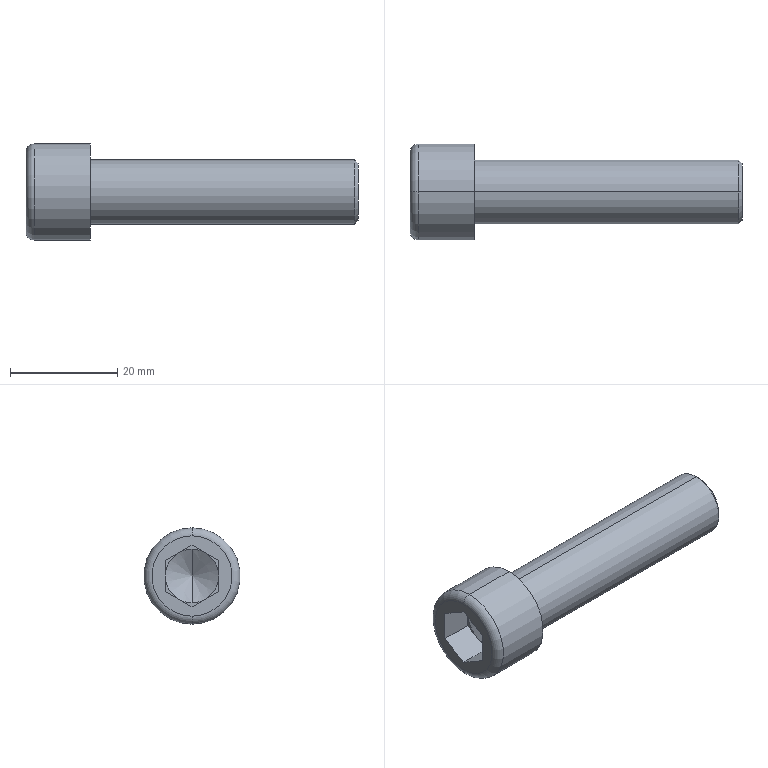Part | STEP file | hexagon socket head cap screws gb_GB_FASTENER_SCREWS_HSHCS M12X50-N | 1 solid | 25 faces | box 62 x 18 x 18 mm | volume 8080 mm3 | plane 15 | cone 4 | cylinder 4 | torus 2 | commonest cylinder face diameters 12 x2 18 x2
STEP:
#1=CARTESIAN_POINT('',(62.,0.,-5.4));
#2=VERTEX_POINT('',#1);
#3=CARTESIAN_POINT('',(62.,0.,5.4));
#4=VERTEX_POINT('',#3);
#5=CARTESIAN_POINT('',(62.,0.,0.));
#6=DIRECTION('',(1.,0.,0.));
#7=DIRECTION('',(0.,0.,-1.));
#8=AXIS2_PLACEMENT_3D('',#5,#6,#7);
#9=CIRCLE('',#8,5.4);
#10=EDGE_CURVE('',#2,#4,#9,.T.);
#11=ORIENTED_EDGE('',*,*,#10,.F.);
#12=CARTESIAN_POINT('',(61.4,0.,-6.));
#13=VERTEX_POINT('',#12);
#14=CARTESIAN_POINT('',(62.,0.,-5.4));
#15=DIRECTION('',(-0.7071,0.,-0.7071));
#16=VECTOR('',#15,1000.);
#17=LINE('',#14,#16);
#18=EDGE_CURVE('',#2,#13,#17,.T.);
#19=ORIENTED_EDGE('',*,*,#18,.T.);
#20=CARTESIAN_POINT('',(61.4,0.,6.));
#21=VERTEX_POINT('',#20);
#22=CARTESIAN_POINT('',(61.4,0.,0.));
#23=DIRECTION('',(-1.,0.,0.));
#24=DIRECTION('',(0.,0.,-1.));
#25=AXIS2_PLACEMENT_3D('',#22,#23,#24);
#26=CIRCLE('',#25,6.);
#27=EDGE_CURVE('',#21,#13,#26,.T.);
#28=ORIENTED_EDGE('',*,*,#27,.F.);
#29=CARTESIAN_POINT('',(62.,0.,5.4));
#30=DIRECTION('',(-0.7071,0.,0.7071));
#31=VECTOR('',#30,1000.);
#32=LINE('',#29,#31);
#33=EDGE_CURVE('',#4,#21,#32,.T.);
#34=ORIENTED_EDGE('',*,*,#33,.F.);
#35=EDGE_LOOP('',(#11,#19,#28,#34));
#36=FACE_OUTER_BOUND('',#35,.T.);
#37=CARTESIAN_POINT('',(62.,0.,0.));
#38=DIRECTION('',(-1.,0.,0.));
#39=DIRECTION('',(0.,0.,1.));
#40=AXIS2_PLACEMENT_3D('',#37,#38,#39);
#41=CONICAL_SURFACE('',#40,5.4,0.7854);
#42=ADVANCED_FACE('',(#36),#41,.T.);
#43=CARTESIAN_POINT('',(0.,0.,7.5));
#44=VERTEX_POINT('',#43);
#45=CARTESIAN_POINT('',(0.,0.,-7.5));
#46=VERTEX_POINT('',#45);
#47=CARTESIAN_POINT('',(0.,0.,0.));
#48=DIRECTION('',(-1.,0.,0.));
#49=DIRECTION('',(0.,0.,-1.));
#50=AXIS2_PLACEMENT_3D('',#47,#48,#49);
#51=CIRCLE('',#50,7.5);
#52=EDGE_CURVE('',#44,#46,#51,.T.);
#53=ORIENTED_EDGE('',*,*,#52,.F.);
#54=CARTESIAN_POINT('',(1.5,0.,9.));
#55=VERTEX_POINT('',#54);
#56=CARTESIAN_POINT('',(1.5,0.,7.5));
#57=DIRECTION('',(0.,1.,0.));
#58=DIRECTION('',(0.,0.,1.));
#59=AXIS2_PLACEMENT_3D('',#56,#57,#58);
#60=CIRCLE('',#59,1.5);
#61=EDGE_CURVE('',#44,#55,#60,.T.);
#62=ORIENTED_EDGE('',*,*,#61,.T.);
#63=CARTESIAN_POINT('',(1.5,0.,-9.));
#64=VERTEX_POINT('',#63);
#65=CARTESIAN_POINT('',(1.5,0.,0.));
#66=DIRECTION('',(1.,0.,0.));
#67=DIRECTION('',(0.,0.,-1.));
#68=AXIS2_PLACEMENT_3D('',#65,#66,#67);
#69=CIRCLE('',#68,9.);
#70=EDGE_CURVE('',#64,#55,#69,.T.);
#71=ORIENTED_EDGE('',*,*,#70,.F.);
#72=CARTESIAN_POINT('',(1.5,0.,-7.5));
#73=DIRECTION('',(0.,-1.,0.));
#74=DIRECTION('',(0.,0.,-1.));
#75=AXIS2_PLACEMENT_3D('',#72,#73,#74);
#76=CIRCLE('',#75,1.5);
#77=EDGE_CURVE('',#46,#64,#76,.T.);
#78=ORIENTED_EDGE('',*,*,#77,.F.);
#79=EDGE_LOOP('',(#53,#62,#71,#78));
#80=FACE_OUTER_BOUND('',#79,.T.);
#81=CARTESIAN_POINT('',(1.5,0.,0.));
#82=DIRECTION('',(1.,0.,0.));
#83=DIRECTION('',(0.,0.,-1.));
#84=AXIS2_PLACEMENT_3D('',#81,#82,#83);
#85=TOROIDAL_SURFACE('',#84,7.5,1.5);
#86=ADVANCED_FACE('',(#80),#85,.T.);
#87=CARTESIAN_POINT('',(8.887,0.,0.));
#88=VERTEX_POINT('',#87);
#89=CARTESIAN_POINT('',(6.,0.,5.));
#90=VERTEX_POINT('',#89);
#91=CARTESIAN_POINT('',(6.,0.,5.));
#92=DIRECTION('',(-0.5,0.,0.866));
#93=VECTOR('',#92,1000.);
#94=LINE('',#91,#93);
#95=EDGE_CURVE('',#88,#90,#94,.T.);
#96=ORIENTED_EDGE('',*,*,#95,.F.);
#97=CARTESIAN_POINT('',(6.,0.,-5.));
#98=VERTEX_POINT('',#97);
#99=CARTESIAN_POINT('',(6.,0.,-5.));
#100=DIRECTION('',(-0.5,0.,-0.866));
#101=VECTOR('',#100,1000.);
#102=LINE('',#99,#101);
#103=EDGE_CURVE('',#88,#98,#102,.T.);
#104=ORIENTED_EDGE('',*,*,#103,.T.);
#105=CARTESIAN_POINT('',(6.,-2.5,-4.33));
#106=VERTEX_POINT('',#105);
#107=CARTESIAN_POINT('',(6.,0.,0.));
#108=DIRECTION('',(-1.,0.,0.));
#109=DIRECTION('',(0.,0.,-1.));
#110=AXIS2_PLACEMENT_3D('',#107,#108,#109);
#111=CIRCLE('',#110,5.);
#112=EDGE_CURVE('',#98,#106,#111,.T.);
#113=ORIENTED_EDGE('',*,*,#112,.T.);
#114=CARTESIAN_POINT('',(6.,-5.,0.));
#115=VERTEX_POINT('',#114);
#116=CARTESIAN_POINT('',(6.,0.,0.));
#117=DIRECTION('',(-1.,0.,0.));
#118=DIRECTION('',(0.,0.,-1.));
#119=AXIS2_PLACEMENT_3D('',#116,#117,#118);
#120=CIRCLE('',#119,5.);
#121=EDGE_CURVE('',#106,#115,#120,.T.);
#122=ORIENTED_EDGE('',*,*,#121,.T.);
#123=CARTESIAN_POINT('',(6.,-2.5,4.33));
#124=VERTEX_POINT('',#123);
#125=CARTESIAN_POINT('',(6.,0.,0.));
#126=DIRECTION('',(-1.,0.,0.));
#127=DIRECTION('',(0.,0.,-1.));
#128=AXIS2_PLACEMENT_3D('',#125,#126,#127);
#129=CIRCLE('',#128,5.);
#130=EDGE_CURVE('',#115,#124,#129,.T.);
#131=ORIENTED_EDGE('',*,*,#130,.T.);
#132=CARTESIAN_POINT('',(6.,0.,0.));
#133=DIRECTION('',(-1.,0.,0.));
#134=DIRECTION('',(0.,0.,-1.));
#135=AXIS2_PLACEMENT_3D('',#132,#133,#134);
#136=CIRCLE('',#135,5.);
#137=EDGE_CURVE('',#124,#90,#136,.T.);
#138=ORIENTED_EDGE('',*,*,#137,.T.);
#139=EDGE_LOOP('',(#96,#104,#113,#122,#131,#138));
#140=FACE_OUTER_BOUND('',#139,.T.);
#141=CARTESIAN_POINT('',(6.,0.,0.));
#142=DIRECTION('',(-1.,0.,0.));
#143=DIRECTION('',(0.,0.,1.));
#144=AXIS2_PLACEMENT_3D('',#141,#142,#143);
#145=CONICAL_SURFACE('',#144,5.,1.047);
#146=ADVANCED_FACE('',(#140),#145,.F.);
#147=ORIENTED_EDGE('',*,*,#27,.T.);
#148=CARTESIAN_POINT('',(12.,0.,-6.));
#149=VERTEX_POINT('',#148);
#150=CARTESIAN_POINT('',(62.,0.,-6.));
#151=DIRECTION('',(-1.,0.,0.));
#152=VECTOR('',#151,1000.);
#153=LINE('',#150,#152);
#154=EDGE_CURVE('',#13,#149,#153,.T.);
#155=ORIENTED_EDGE('',*,*,#154,.T.);
#156=CARTESIAN_POINT('',(12.,0.,6.));
#157=VERTEX_POINT('',#156);
#158=CARTESIAN_POINT('',(12.,0.,0.));
#159=DIRECTION('',(1.,0.,0.));
#160=DIRECTION('',(0.,0.,-1.));
#161=AXIS2_PLACEMENT_3D('',#158,#159,#160);
#162=CIRCLE('',#161,6.);
#163=EDGE_CURVE('',#149,#157,#162,.T.);
#164=ORIENTED_EDGE('',*,*,#163,.T.);
#165=CARTESIAN_POINT('',(62.,0.,6.));
#166=DIRECTION('',(-1.,0.,0.));
#167=VECTOR('',#166,1000.);
#168=LINE('',#165,#167);
#169=EDGE_CURVE('',#21,#157,#168,.T.);
#170=ORIENTED_EDGE('',*,*,#169,.F.);
#171=EDGE_LOOP('',(#147,#155,#164,#170));
#172=FACE_OUTER_BOUND('',#171,.T.);
#173=CARTESIAN_POINT('',(62.,0.,0.));
#174=DIRECTION('',(-1.,0.,0.));
#175=DIRECTION('',(0.,0.,1.));
#176=AXIS2_PLACEMENT_3D('',#173,#174,#175);
#177=CYLINDRICAL_SURFACE('',#176,6.);
#178=ADVANCED_FACE('',(#172),#177,.T.);
#179=CARTESIAN_POINT('',(12.,0.,-9.));
#180=VERTEX_POINT('',#179);
#181=CARTESIAN_POINT('',(12.,0.,9.));
#182=VERTEX_POINT('',#181);
#183=CARTESIAN_POINT('',(12.,0.,0.));
#184=DIRECTION('',(1.,0.,0.));
#185=DIRECTION('',(0.,0.,-1.));
#186=AXIS2_PLACEMENT_3D('',#183,#184,#185);
#187=CIRCLE('',#186,9.);
#188=EDGE_CURVE('',#180,#182,#187,.T.);
#189=ORIENTED_EDGE('',*,*,#188,.F.);
#190=CARTESIAN_POINT('',(12.,0.,-9.));
#191=DIRECTION('',(-1.,0.,0.));
#192=VECTOR('',#191,1000.);
#193=LINE('',#190,#192);
#194=EDGE_CURVE('',#180,#64,#193,.T.);
#195=ORIENTED_EDGE('',*,*,#194,.T.);
#196=ORIENTED_EDGE('',*,*,#70,.T.);
#197=CARTESIAN_POINT('',(12.,0.,9.));
#198=DIRECTION('',(-1.,0.,0.));
#199=VECTOR('',#198,1000.);
#200=LINE('',#197,#199);
#201=EDGE_CURVE('',#182,#55,#200,.T.);
#202=ORIENTED_EDGE('',*,*,#201,.F.);
#203=EDGE_LOOP('',(#189,#195,#196,#202));
#204=FACE_OUTER_BOUND('',#203,.T.);
#205=CARTESIAN_POINT('',(12.,0.,0.));
#206=DIRECTION('',(-1.,0.,0.));
#207=DIRECTION('',(0.,0.,1.));
#208=AXIS2_PLACEMENT_3D('',#205,#206,#207);
#209=CYLINDRICAL_SURFACE('',#208,9.);
#210=ADVANCED_FACE('',(#204),#209,.T.);
#211=ORIENTED_EDGE('',*,*,#121,.F.);
#212=CARTESIAN_POINT('',(6.,-5.,-2.887));
#213=VERTEX_POINT('',#212);
#214=CARTESIAN_POINT('',(6.,-5.,-2.887));
#215=DIRECTION('',(0.,0.866,-0.5));
#216=VECTOR('',#215,1000.);
#217=LINE('',#214,#216);
#218=EDGE_CURVE('',#213,#106,#217,.T.);
#219=ORIENTED_EDGE('',*,*,#218,.F.);
#220=CARTESIAN_POINT('',(6.,-5.,2.887));
#221=DIRECTION('',(0.,0.,-1.));
#222=VECTOR('',#221,1000.);
#223=LINE('',#220,#222);
#224=EDGE_CURVE('',#115,#213,#223,.T.);
#225=ORIENTED_EDGE('',*,*,#224,.F.);
#226=EDGE_LOOP('',(#211,#219,#225));
#227=FACE_OUTER_BOUND('',#226,.T.);
#228=CARTESIAN_POINT('',(6.,0.,-5.774));
#229=DIRECTION('',(1.,0.,0.));
#230=DIRECTION('',(0.,0.,-1.));
#231=AXIS2_PLACEMENT_3D('',#228,#229,#230);
#232=PLANE('',#231);
#233=ADVANCED_FACE('',(#227),#232,.F.);
#234=ORIENTED_EDGE('',*,*,#130,.F.);
#235=CARTESIAN_POINT('',(6.,-5.,2.887));
#236=VERTEX_POINT('',#235);
#237=CARTESIAN_POINT('',(6.,-5.,2.887));
#238=DIRECTION('',(0.,0.,-1.));
#239=VECTOR('',#238,1000.);
#240=LINE('',#237,#239);
#241=EDGE_CURVE('',#236,#115,#240,.T.);
#242=ORIENTED_EDGE('',*,*,#241,.F.);
#243=CARTESIAN_POINT('',(6.,0.,5.774));
#244=DIRECTION('',(0.,-0.866,-0.5));
#245=VECTOR('',#244,1000.);
#246=LINE('',#243,#245);
#247=EDGE_CURVE('',#124,#236,#246,.T.);
#248=ORIENTED_EDGE('',*,*,#247,.F.);
#249=EDGE_LOOP('',(#234,#242,#248));
#250=FACE_OUTER_BOUND('',#249,.T.);
#251=CARTESIAN_POINT('',(6.,0.,-5.774));
#252=DIRECTION('',(1.,0.,0.));
#253=DIRECTION('',(0.,0.,-1.));
#254=AXIS2_PLACEMENT_3D('',#251,#252,#253);
#255=PLANE('',#254);
#256=ADVANCED_FACE('',(#250),#255,.F.);
#257=ORIENTED_EDGE('',*,*,#137,.F.);
#258=CARTESIAN_POINT('',(6.,0.,5.774));
#259=VERTEX_POINT('',#258);
#260=CARTESIAN_POINT('',(6.,0.,5.774));
#261=DIRECTION('',(0.,-0.866,-0.5));
#262=VECTOR('',#261,1000.);
#263=LINE('',#260,#262);
#264=EDGE_CURVE('',#259,#124,#263,.T.);
#265=ORIENTED_EDGE('',*,*,#264,.F.);
#266=CARTESIAN_POINT('',(6.,2.5,4.33));
#267=VERTEX_POINT('',#266);
#268=CARTESIAN_POINT('',(6.,5.,2.887));
#269=DIRECTION('',(0.,-0.866,0.5));
#270=VECTOR('',#269,1000.);
#271=LINE('',#268,#270);
#272=EDGE_CURVE('',#267,#259,#271,.T.);
#273=ORIENTED_EDGE('',*,*,#272,.F.);
#274=CARTESIAN_POINT('',(6.,0.,0.));
#275=DIRECTION('',(-1.,0.,0.));
#276=DIRECTION('',(0.,0.,-1.));
#277=AXIS2_PLACEMENT_3D('',#274,#275,#276);
#278=CIRCLE('',#277,5.);
#279=EDGE_CURVE('',#90,#267,#278,.T.);
#280=ORIENTED_EDGE('',*,*,#279,.F.);
#281=EDGE_LOOP('',(#257,#265,#273,#280));
#282=FACE_OUTER_BOUND('',#281,.T.);
#283=CARTESIAN_POINT('',(6.,0.,-5.774));
#284=DIRECTION('',(1.,0.,0.));
#285=DIRECTION('',(0.,0.,-1.));
#286=AXIS2_PLACEMENT_3D('',#283,#284,#285);
#287=PLANE('',#286);
#288=ADVANCED_FACE('',(#282),#287,.F.);
#289=CARTESIAN_POINT('',(6.,5.,0.));
#290=VERTEX_POINT('',#289);
#291=CARTESIAN_POINT('',(6.,0.,0.));
#292=DIRECTION('',(-1.,0.,0.));
#293=DIRECTION('',(0.,0.,-1.));
#294=AXIS2_PLACEMENT_3D('',#291,#292,#293);
#295=CIRCLE('',#294,5.);
#296=EDGE_CURVE('',#267,#290,#295,.T.);
#297=ORIENTED_EDGE('',*,*,#296,.F.);
#298=CARTESIAN_POINT('',(6.,5.,2.887));
#299=VERTEX_POINT('',#298);
#300=CARTESIAN_POINT('',(6.,5.,2.887));
#301=DIRECTION('',(0.,-0.866,0.5));
#302=VECTOR('',#301,1000.);
#303=LINE('',#300,#302);
#304=EDGE_CURVE('',#299,#267,#303,.T.);
#305=ORIENTED_EDGE('',*,*,#304,.F.);
#306=CARTESIAN_POINT('',(6.,5.,-2.887));
#307=DIRECTION('',(0.,0.,1.));
#308=VECTOR('',#307,1000.);
#309=LINE('',#306,#308);
#310=EDGE_CURVE('',#290,#299,#309,.T.);
#311=ORIENTED_EDGE('',*,*,#310,.F.);
#312=EDGE_LOOP('',(#297,#305,#311));
#313=FACE_OUTER_BOUND('',#312,.T.);
#314=CARTESIAN_POINT('',(6.,0.,-5.774));
#315=DIRECTION('',(1.,0.,0.));
#316=DIRECTION('',(0.,0.,-1.));
#317=AXIS2_PLACEMENT_3D('',#314,#315,#316);
#318=PLANE('',#317);
#319=ADVANCED_FACE('',(#313),#318,.F.);
#320=CARTESIAN_POINT('',(6.,2.5,-4.33));
#321=VERTEX_POINT('',#320);
#322=CARTESIAN_POINT('',(6.,0.,0.));
#323=DIRECTION('',(1.,0.,0.));
#324=DIRECTION('',(0.,0.,-1.));
#325=AXIS2_PLACEMENT_3D('',#322,#323,#324);
#326=CIRCLE('',#325,5.);
#327=EDGE_CURVE('',#321,#290,#326,.T.);
#328=ORIENTED_EDGE('',*,*,#327,.T.);
#329=CARTESIAN_POINT('',(6.,5.,-2.887));
#330=VERTEX_POINT('',#329);
#331=CARTESIAN_POINT('',(6.,5.,-2.887));
#332=DIRECTION('',(0.,0.,1.));
#333=VECTOR('',#332,1000.);
#334=LINE('',#331,#333);
#335=EDGE_CURVE('',#330,#290,#334,.T.);
#336=ORIENTED_EDGE('',*,*,#335,.F.);
#337=CARTESIAN_POINT('',(6.,0.,-5.774));
#338=DIRECTION('',(0.,0.866,0.5));
#339=VECTOR('',#338,1000.);
#340=LINE('',#337,#339);
#341=EDGE_CURVE('',#321,#330,#340,.T.);
#342=ORIENTED_EDGE('',*,*,#341,.F.);
#343=EDGE_LOOP('',(#328,#336,#342));
#344=FACE_OUTER_BOUND('',#343,.T.);
#345=CARTESIAN_POINT('',(6.,0.,-5.774));
#346=DIRECTION('',(1.,0.,0.));
#347=DIRECTION('',(0.,0.,-1.));
#348=AXIS2_PLACEMENT_3D('',#345,#346,#347);
#349=PLANE('',#348);
#350=ADVANCED_FACE('',(#344),#349,.F.);
#351=CARTESIAN_POINT('',(6.,0.,0.));
#352=DIRECTION('',(-1.,0.,0.));
#353=DIRECTION('',(0.,0.,-1.));
#354=AXIS2_PLACEMENT_3D('',#351,#352,#353);
#355=CIRCLE('',#354,5.);
#356=EDGE_CURVE('',#321,#98,#355,.T.);
#357=ORIENTED_EDGE('',*,*,#356,.F.);
#358=CARTESIAN_POINT('',(6.,0.,-5.774));
#359=VERTEX_POINT('',#358);
#360=CARTESIAN_POINT('',(6.,0.,-5.774));
#361=DIRECTION('',(0.,0.866,0.5));
#362=VECTOR('',#361,1000.);
#363=LINE('',#360,#362);
#364=EDGE_CURVE('',#359,#321,#363,.T.);
#365=ORIENTED_EDGE('',*,*,#364,.F.);
#366=CARTESIAN_POINT('',(6.,-5.,-2.887));
#367=DIRECTION('',(0.,0.866,-0.5));
#368=VECTOR('',#367,1000.);
#369=LINE('',#366,#368);
#370=EDGE_CURVE('',#106,#359,#369,.T.);
#371=ORIENTED_EDGE('',*,*,#370,.F.);
#372=ORIENTED_EDGE('',*,*,#112,.F.);
#373=EDGE_LOOP('',(#357,#365,#371,#372));
#374=FACE_OUTER_BOUND('',#373,.T.);
#375=CARTESIAN_POINT('',(6.,0.,-5.774));
#376=DIRECTION('',(1.,0.,0.));
#377=DIRECTION('',(0.,0.,-1.));
#378=AXIS2_PLACEMENT_3D('',#375,#376,#377);
#379=PLANE('',#378);
#380=ADVANCED_FACE('',(#374),#379,.F.);
#381=CARTESIAN_POINT('',(0.,0.,0.));
#382=DIRECTION('',(-1.,0.,0.));
#383=DIRECTION('',(0.,0.,-1.));
#384=AXIS2_PLACEMENT_3D('',#381,#382,#383);
#385=CIRCLE('',#384,7.5);
#386=EDGE_CURVE('',#46,#44,#385,.T.);
#387=ORIENTED_EDGE('',*,*,#386,.T.);
#388=ORIENTED_EDGE('',*,*,#52,.T.);
#389=EDGE_LOOP('',(#387,#388));
#390=FACE_OUTER_BOUND('',#389,.T.);
#391=CARTESIAN_POINT('',(0.,-5.,-2.887));
#392=VERTEX_POINT('',#391);
#393=CARTESIAN_POINT('',(0.,0.,-5.774));
#394=VERTEX_POINT('',#393);
#395=CARTESIAN_POINT('',(0.,-5.,-2.887));
#396=DIRECTION('',(0.,0.866,-0.5));
#397=VECTOR('',#396,1000.);
#398=LINE('',#395,#397);
#399=EDGE_CURVE('',#392,#394,#398,.T.);
#400=ORIENTED_EDGE('',*,*,#399,.T.);
#401=CARTESIAN_POINT('',(0.,5.,-2.887));
#402=VERTEX_POINT('',#401);
#403=CARTESIAN_POINT('',(0.,0.,-5.774));
#404=DIRECTION('',(0.,0.866,0.5));
#405=VECTOR('',#404,1000.);
#406=LINE('',#403,#405);
#407=EDGE_CURVE('',#394,#402,#406,.T.);
#408=ORIENTED_EDGE('',*,*,#407,.T.);
#409=CARTESIAN_POINT('',(0.,5.,2.887));
#410=VERTEX_POINT('',#409);
#411=CARTESIAN_POINT('',(0.,5.,-2.887));
#412=DIRECTION('',(0.,0.,1.));
#413=VECTOR('',#412,1000.);
#414=LINE('',#411,#413);
#415=EDGE_CURVE('',#402,#410,#414,.T.);
#416=ORIENTED_EDGE('',*,*,#415,.T.);
#417=CARTESIAN_POINT('',(0.,0.,5.774));
#418=VERTEX_POINT('',#417);
#419=CARTESIAN_POINT('',(0.,5.,2.887));
#420=DIRECTION('',(0.,-0.866,0.5));
#421=VECTOR('',#420,1000.);
#422=LINE('',#419,#421);
#423=EDGE_CURVE('',#410,#418,#422,.T.);
#424=ORIENTED_EDGE('',*,*,#423,.T.);
#425=CARTESIAN_POINT('',(0.,-5.,2.887));
#426=VERTEX_POINT('',#425);
#427=CARTESIAN_POINT('',(0.,0.,5.774));
#428=DIRECTION('',(0.,-0.866,-0.5));
#429=VECTOR('',#428,1000.);
#430=LINE('',#427,#429);
#431=EDGE_CURVE('',#418,#426,#430,.T.);
#432=ORIENTED_EDGE('',*,*,#431,.T.);
#433=CARTESIAN_POINT('',(0.,-5.,2.887));
#434=DIRECTION('',(0.,0.,-1.));
#435=VECTOR('',#434,1000.);
#436=LINE('',#433,#435);
#437=EDGE_CURVE('',#426,#392,#436,.T.);
#438=ORIENTED_EDGE('',*,*,#437,.T.);
#439=EDGE_LOOP('',(#400,#408,#416,#424,#432,#438));
#440=FACE_BOUND('',#439,.T.);
#441=CARTESIAN_POINT('',(0.,0.,0.));
#442=DIRECTION('',(1.,0.,0.));
#443=DIRECTION('',(0.,0.,-1.));
#444=AXIS2_PLACEMENT_3D('',#441,#442,#443);
#445=PLANE('',#444);
#446=ADVANCED_FACE('',(#390,#440),#445,.F.);
#447=CARTESIAN_POINT('',(12.,0.,0.));
#448=DIRECTION('',(1.,0.,0.));
#449=DIRECTION('',(0.,0.,-1.));
#450=AXIS2_PLACEMENT_3D('',#447,#448,#449);
#451=CIRCLE('',#450,9.);
#452=EDGE_CURVE('',#182,#180,#451,.T.);
#453=ORIENTED_EDGE('',*,*,#452,.T.);
#454=ORIENTED_EDGE('',*,*,#188,.T.);
#455=EDGE_LOOP('',(#453,#454));
#456=FACE_OUTER_BOUND('',#455,.T.);
#457=CARTESIAN_POINT('',(12.,0.,0.));
#458=DIRECTION('',(1.,0.,0.));
#459=DIRECTION('',(0.,0.,-1.));
#460=AXIS2_PLACEMENT_3D('',#457,#458,#459);
#461=CIRCLE('',#460,6.);
#462=EDGE_CURVE('',#157,#149,#461,.T.);
#463=ORIENTED_EDGE('',*,*,#462,.F.);
#464=ORIENTED_EDGE('',*,*,#163,.F.);
#465=EDGE_LOOP('',(#463,#464));
#466=FACE_BOUND('',#465,.T.);
#467=CARTESIAN_POINT('',(12.,0.,0.));
#468=DIRECTION('',(1.,0.,0.));
#469=DIRECTION('',(0.,0.,-1.));
#470=AXIS2_PLACEMENT_3D('',#467,#468,#469);
#471=PLANE('',#470);
#472=ADVANCED_FACE('',(#456,#466),#471,.T.);
#473=ORIENTED_EDGE('',*,*,#194,.F.);
#474=ORIENTED_EDGE('',*,*,#452,.F.);
#475=ORIENTED_EDGE('',*,*,#201,.T.);
#476=CARTESIAN_POINT('',(1.5,0.,0.));
#477=DIRECTION('',(1.,0.,0.));
#478=DIRECTION('',(0.,0.,-1.));
#479=AXIS2_PLACEMENT_3D('',#476,#477,#478);
#480=CIRCLE('',#479,9.);
#481=EDGE_CURVE('',#55,#64,#480,.T.);
#482=ORIENTED_EDGE('',*,*,#481,.T.);
#483=EDGE_LOOP('',(#473,#474,#475,#482));
#484=FACE_OUTER_BOUND('',#483,.T.);
#485=CARTESIAN_POINT('',(12.,0.,0.));
#486=DIRECTION('',(-1.,0.,0.));
#487=DIRECTION('',(0.,0.,1.));
#488=AXIS2_PLACEMENT_3D('',#485,#486,#487);
#489=CYLINDRICAL_SURFACE('',#488,9.);
#490=ADVANCED_FACE('',(#484),#489,.T.);
#491=ORIENTED_EDGE('',*,*,#154,.F.);
#492=CARTESIAN_POINT('',(61.4,0.,0.));
#493=DIRECTION('',(-1.,0.,0.));
#494=DIRECTION('',(0.,0.,-1.));
#495=AXIS2_PLACEMENT_3D('',#492,#493,#494);
#496=CIRCLE('',#495,6.);
#497=EDGE_CURVE('',#13,#21,#496,.T.);
#498=ORIENTED_EDGE('',*,*,#497,.T.);
#499=ORIENTED_EDGE('',*,*,#169,.T.);
#500=ORIENTED_EDGE('',*,*,#462,.T.);
#501=EDGE_LOOP('',(#491,#498,#499,#500));
#502=FACE_OUTER_BOUND('',#501,.T.);
#503=CARTESIAN_POINT('',(62.,0.,0.));
#504=DIRECTION('',(-1.,0.,0.));
#505=DIRECTION('',(0.,0.,1.));
#506=AXIS2_PLACEMENT_3D('',#503,#504,#505);
#507=CYLINDRICAL_SURFACE('',#506,6.);
#508=ADVANCED_FACE('',(#502),#507,.T.);
#509=CARTESIAN_POINT('',(62.,0.,0.));
#510=DIRECTION('',(1.,0.,0.));
#511=DIRECTION('',(0.,0.,-1.));
#512=AXIS2_PLACEMENT_3D('',#509,#510,#511);
#513=CIRCLE('',#512,5.4);
#514=EDGE_CURVE('',#4,#2,#513,.T.);
#515=ORIENTED_EDGE('',*,*,#514,.T.);
#516=ORIENTED_EDGE('',*,*,#10,.T.);
#517=EDGE_LOOP('',(#515,#516));
#518=FACE_OUTER_BOUND('',#517,.T.);
#519=CARTESIAN_POINT('',(62.,0.,0.));
#520=DIRECTION('',(1.,0.,0.));
#521=DIRECTION('',(0.,0.,-1.));
#522=AXIS2_PLACEMENT_3D('',#519,#520,#521);
#523=PLANE('',#522);
#524=ADVANCED_FACE('',(#518),#523,.T.);
#525=ORIENTED_EDGE('',*,*,#399,.F.);
#526=CARTESIAN_POINT('',(6.,-5.,-2.887));
#527=DIRECTION('',(-1.,0.,0.));
#528=VECTOR('',#527,1000.);
#529=LINE('',#526,#528);
#530=EDGE_CURVE('',#213,#392,#529,.T.);
#531=ORIENTED_EDGE('',*,*,#530,.F.);
#532=ORIENTED_EDGE('',*,*,#218,.T.);
#533=ORIENTED_EDGE('',*,*,#370,.T.);
#534=CARTESIAN_POINT('',(6.,0.,-5.774));
#535=DIRECTION('',(-1.,0.,0.));
#536=VECTOR('',#535,1000.);
#537=LINE('',#534,#536);
#538=EDGE_CURVE('',#359,#394,#537,.T.);
#539=ORIENTED_EDGE('',*,*,#538,.T.);
#540=EDGE_LOOP('',(#525,#531,#532,#533,#539));
#541=FACE_OUTER_BOUND('',#540,.T.);
#542=CARTESIAN_POINT('',(6.,-5.,-2.887));
#543=DIRECTION('',(0.,0.5,0.866));
#544=DIRECTION('',(0.,-0.866,0.5));
#545=AXIS2_PLACEMENT_3D('',#542,#543,#544);
#546=PLANE('',#545);
#547=ADVANCED_FACE('',(#541),#546,.T.);
#548=ORIENTED_EDGE('',*,*,#407,.F.);
#549=ORIENTED_EDGE('',*,*,#538,.F.);
#550=ORIENTED_EDGE('',*,*,#364,.T.);
#551=ORIENTED_EDGE('',*,*,#341,.T.);
#552=CARTESIAN_POINT('',(6.,5.,-2.887));
#553=DIRECTION('',(-1.,0.,0.));
#554=VECTOR('',#553,1000.);
#555=LINE('',#552,#554);
#556=EDGE_CURVE('',#330,#402,#555,.T.);
#557=ORIENTED_EDGE('',*,*,#556,.T.);
#558=EDGE_LOOP('',(#548,#549,#550,#551,#557));
#559=FACE_OUTER_BOUND('',#558,.T.);
#560=CARTESIAN_POINT('',(6.,0.,-5.774));
#561=DIRECTION('',(0.,-0.5,0.866));
#562=DIRECTION('',(0.,-0.866,-0.5));
#563=AXIS2_PLACEMENT_3D('',#560,#561,#562);
#564=PLANE('',#563);
#565=ADVANCED_FACE('',(#559),#564,.T.);
#566=ORIENTED_EDGE('',*,*,#415,.F.);
#567=ORIENTED_EDGE('',*,*,#556,.F.);
#568=ORIENTED_EDGE('',*,*,#335,.T.);
#569=ORIENTED_EDGE('',*,*,#310,.T.);
#570=CARTESIAN_POINT('',(6.,5.,2.887));
#571=DIRECTION('',(-1.,0.,0.));
#572=VECTOR('',#571,1000.);
#573=LINE('',#570,#572);
#574=EDGE_CURVE('',#299,#410,#573,.T.);
#575=ORIENTED_EDGE('',*,*,#574,.T.);
#576=EDGE_LOOP('',(#566,#567,#568,#569,#575));
#577=FACE_OUTER_BOUND('',#576,.T.);
#578=CARTESIAN_POINT('',(6.,5.,-2.887));
#579=DIRECTION('',(0.,-1.,0.));
#580=DIRECTION('',(0.,0.,-1.));
#581=AXIS2_PLACEMENT_3D('',#578,#579,#580);
#582=PLANE('',#581);
#583=ADVANCED_FACE('',(#577),#582,.T.);
#584=ORIENTED_EDGE('',*,*,#423,.F.);
#585=ORIENTED_EDGE('',*,*,#574,.F.);
#586=ORIENTED_EDGE('',*,*,#304,.T.);
#587=ORIENTED_EDGE('',*,*,#272,.T.);
#588=CARTESIAN_POINT('',(6.,0.,5.774));
#589=DIRECTION('',(-1.,0.,0.));
#590=VECTOR('',#589,1000.);
#591=LINE('',#588,#590);
#592=EDGE_CURVE('',#259,#418,#591,.T.);
#593=ORIENTED_EDGE('',*,*,#592,.T.);
#594=EDGE_LOOP('',(#584,#585,#586,#587,#593));
#595=FACE_OUTER_BOUND('',#594,.T.);
#596=CARTESIAN_POINT('',(6.,5.,2.887));
#597=DIRECTION('',(0.,-0.5,-0.866));
#598=DIRECTION('',(0.,0.866,-0.5));
#599=AXIS2_PLACEMENT_3D('',#596,#597,#598);
#600=PLANE('',#599);
#601=ADVANCED_FACE('',(#595),#600,.T.);
#602=ORIENTED_EDGE('',*,*,#431,.F.);
#603=ORIENTED_EDGE('',*,*,#592,.F.);
#604=ORIENTED_EDGE('',*,*,#264,.T.);
#605=ORIENTED_EDGE('',*,*,#247,.T.);
#606=CARTESIAN_POINT('',(6.,-5.,2.887));
#607=DIRECTION('',(-1.,0.,0.));
#608=VECTOR('',#607,1000.);
#609=LINE('',#606,#608);
#610=EDGE_CURVE('',#236,#426,#609,.T.);
#611=ORIENTED_EDGE('',*,*,#610,.T.);
#612=EDGE_LOOP('',(#602,#603,#604,#605,#611));
#613=FACE_OUTER_BOUND('',#612,.T.);
#614=CARTESIAN_POINT('',(6.,0.,5.774));
#615=DIRECTION('',(0.,0.5,-0.866));
#616=DIRECTION('',(0.,0.866,0.5));
#617=AXIS2_PLACEMENT_3D('',#614,#615,#616);
#618=PLANE('',#617);
#619=ADVANCED_FACE('',(#613),#618,.T.);
#620=ORIENTED_EDGE('',*,*,#437,.F.);
#621=ORIENTED_EDGE('',*,*,#610,.F.);
#622=ORIENTED_EDGE('',*,*,#241,.T.);
#623=ORIENTED_EDGE('',*,*,#224,.T.);
#624=ORIENTED_EDGE('',*,*,#530,.T.);
#625=EDGE_LOOP('',(#620,#621,#622,#623,#624));
#626=FACE_OUTER_BOUND('',#625,.T.);
#627=CARTESIAN_POINT('',(6.,-5.,2.887));
#628=DIRECTION('',(0.,1.,0.));
#629=DIRECTION('',(0.,0.,1.));
#630=AXIS2_PLACEMENT_3D('',#627,#628,#629);
#631=PLANE('',#630);
#632=ADVANCED_FACE('',(#626),#631,.T.);
#633=ORIENTED_EDGE('',*,*,#103,.F.);
#634=ORIENTED_EDGE('',*,*,#95,.T.);
#635=ORIENTED_EDGE('',*,*,#279,.T.);
#636=ORIENTED_EDGE('',*,*,#296,.T.);
#637=ORIENTED_EDGE('',*,*,#327,.F.);
#638=ORIENTED_EDGE('',*,*,#356,.T.);
#639=EDGE_LOOP('',(#633,#634,#635,#636,#637,#638));
#640=FACE_OUTER_BOUND('',#639,.T.);
#641=CARTESIAN_POINT('',(6.,0.,0.));
#642=DIRECTION('',(-1.,0.,0.));
#643=DIRECTION('',(0.,0.,1.));
#644=AXIS2_PLACEMENT_3D('',#641,#642,#643);
#645=CONICAL_SURFACE('',#644,5.,1.047);
#646=ADVANCED_FACE('',(#640),#645,.F.);
#647=ORIENTED_EDGE('',*,*,#61,.F.);
#648=ORIENTED_EDGE('',*,*,#386,.F.);
#649=ORIENTED_EDGE('',*,*,#77,.T.);
#650=ORIENTED_EDGE('',*,*,#481,.F.);
#651=EDGE_LOOP('',(#647,#648,#649,#650));
#652=FACE_OUTER_BOUND('',#651,.T.);
#653=CARTESIAN_POINT('',(1.5,0.,0.));
#654=DIRECTION('',(1.,0.,0.));
#655=DIRECTION('',(0.,0.,-1.));
#656=AXIS2_PLACEMENT_3D('',#653,#654,#655);
#657=TOROIDAL_SURFACE('',#656,7.5,1.5);
#658=ADVANCED_FACE('',(#652),#657,.T.);
#659=ORIENTED_EDGE('',*,*,#18,.F.);
#660=ORIENTED_EDGE('',*,*,#514,.F.);
#661=ORIENTED_EDGE('',*,*,#33,.T.);
#662=ORIENTED_EDGE('',*,*,#497,.F.);
#663=EDGE_LOOP('',(#659,#660,#661,#662));
#664=FACE_OUTER_BOUND('',#663,.T.);
#665=CARTESIAN_POINT('',(62.,0.,0.));
#666=DIRECTION('',(-1.,0.,0.));
#667=DIRECTION('',(0.,0.,1.));
#668=AXIS2_PLACEMENT_3D('',#665,#666,#667);
#669=CONICAL_SURFACE('',#668,5.4,0.7854);
#670=ADVANCED_FACE('',(#664),#669,.T.);
#671=CLOSED_SHELL('',(#42,#86,#146,#178,#210,#233,#256,#288,#319,#350,#380,#446,#472,#490,#508,#524,#547,#565,#583,#601,#619,#632,#646,#658,#670));
#672=MANIFOLD_SOLID_BREP('',#671);
#673=CARTESIAN_POINT('',(0.,0.,0.));
#674=DIRECTION('',(0.,0.,1.));
#675=DIRECTION('',(1.,0.,0.));
#676=AXIS2_PLACEMENT_3D('',#673,#674,#675);
#677=(LENGTH_UNIT()NAMED_UNIT(*)SI_UNIT(.MILLI.,.METRE.));
#678=UNCERTAINTY_MEASURE_WITH_UNIT(LENGTH_MEASURE(0.00001),#677,'','');
#679=(NAMED_UNIT(*)PLANE_ANGLE_UNIT()SI_UNIT($,.RADIAN.));
#680=(NAMED_UNIT(*)SI_UNIT($,.STERADIAN.)SOLID_ANGLE_UNIT());
#681=(GEOMETRIC_REPRESENTATION_CONTEXT(3)GLOBAL_UNCERTAINTY_ASSIGNED_CONTEXT((#678))GLOBAL_UNIT_ASSIGNED_CONTEXT((#677,#679,#680))REPRESENTATION_CONTEXT('',''));
#682=ADVANCED_BREP_SHAPE_REPRESENTATION('',(#672,#676),#681);